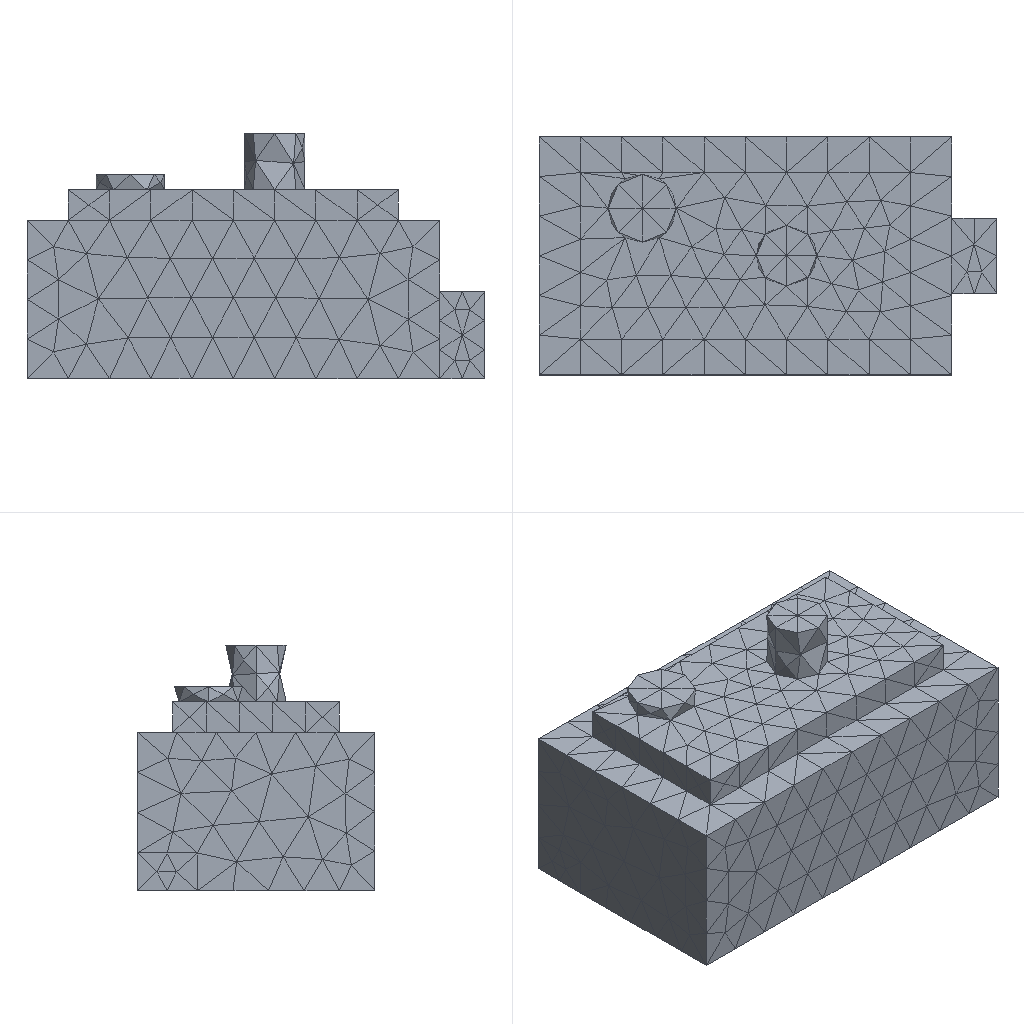Simulation study | ansys mapdl
Set-up summary:
category,name,step,type,value,unit,region
solver,ansys_mapdl
units,mm-N-s-tonne (MPa),,inferred,E=210000 density=
analysis,model,,static
mesh,nodes,,,4621
mesh,elements,,,2783
element_type,SOLID187,,,2783
material,mat 1,,E,210000
material,mat 1,,nu,0.3
load,,model,body load temp,,,all
load,,model,force,"1000 [dir=(0, 0, -1) n=138]",,node list
bc,,model,fixed,"[dofs=UX,UY,UZ n=4927]",,node list
Ansys APDL input file, long lists of numbers shortened:
/COM,ANSYS RELEASE 2026 R1           BUILD 26.1      UP20260202       09:08:46
/PREP7
/NOPR
/TITLE,2
ANTYPE, 0
*IF,_CDRDOFF,EQ,1,THEN     !if solid model was read in
_CDRDOFF=             !reset flag, numoffs already performed
*ELSE              !offset database for the following FE model
NUMOFF,NODE,     4621
NUMOFF,ELEM,     2783
NUMOFF,MAT ,        1
NUMOFF,TYPE,        1
*ENDIF
*SET,_RETURN ,  0.
*SET,_STATUS ,  0.
*SET,_UIQR   ,  138.
*SET,__FLOATPARAMETER__,  4621.
DOF,DELETE
ETBLOCK,        1,        1
(2i9,19a9)
        1      187        0        0        0        0        0        0        0        0        0        0        0        0        0        0        0        0        0        0        0
       -1
NBLOCK,6,SOLID,      4621,      4621
(3i9,6e21.13e3)
        1        0        0-3.8625000000000E+001 3.1500000000000E+001 1.0000000000000E+001
! (4620 more lines like these left out)
N,UNBL,LOC,       -1,
EBLOCK,19,SOLID,      2783,      2783
(19i10)
         1         1         1         1         0         0         0         0        10         0         1      1542      1719       451      1720      1993      1994      1995      1996
! (5565 more lines like these left out)
        -1
MPTEMP,UNBL, 1, 1,  0.    ,
MPDATA,UNBL, 1,EX  ,       1, 1,  210000.000    ,
MPTEMP,UNBL, 1, 1,  0.    ,
MPDATA,UNBL, 1,NUXY,       1, 1, 0.3    ,
MPTEMP,UNBL, 1, 1,  0.    ,
MPDATA,UNBL, 1,PRXY,       1, 1, 0.3    ,
EXTOPT,ATTR,      0,      0,      0
EXTOPT,ESIZE,  0,  0.
EXTOPT,ACLEAR,      0
TREF,  0.
IRLF,  0
BFUNIF,TEMP,_TINY
ACEL,  0.    ,  0.    ,  0.
OMEGA,  0.    ,  0.    ,  0.
DOMEGA,  0.    ,  0.    ,  0.
CGLOC,  0.    ,  0.    ,  0.
CGOMEGA,  0.    ,  0.    ,  0.
DCGOMG,  0.    ,  0.    ,  0.
KUSE,     0
TIME,  0.
ALPHAD,  0.
BETAD,  0.
DMPRAT,  0.
DMPSTR,  0.
CRPLIM, 0.1    ,   0
CRPLIM,  0.    ,   1
NCNV,     0, 1.000000000E+12,     0,  0.    ,  0.
NEQIT,     0
ERESX,DEFA
DBLOCK,      4927
(i9,a6,2(pg16.9))
        1  UX    0.00000000      0.00000000
! (4926 more lines like these left out)
       -1
FBLOCK,       138
(i9,a6,2(pg16.9))
      824  FZ   -7.24637681      0.00000000
! (137 more lines like these left out)
       -1
/GO
FINISH
Results summary:
result,analysis_type_db,,,static,unstated
result,n_sets,,,1,unstated
result,load_steps[0].set,load_step=1,,1,unstated
result,load_steps[0].substep,load_step=1,,1,unstated
result,load_steps[0].time,load_step=1,,1,unstated
result,load_steps[0].freq,load_step=1,,1,unstated
result,load_steps[0].max_usum,load_step=1,,0.0004131,unstated
result,load_steps[0].max_seqv,load_step=1,,4.888,unstated
result,load_steps[0].reaction_sum.FX,load_step=1,,1.0969e-11,unstated
result,load_steps[0].reaction_sum.FY,load_step=1,,-1.69153e-11,unstated
result,load_steps[0].reaction_sum.FZ,load_step=1,,1000,unstated
result,load_steps[0].reaction_sum.MX,load_step=1,,0,unstated
result,load_steps[0].reaction_sum.MY,load_step=1,,0,unstated
result,load_steps[0].reaction_sum.MZ,load_step=1,,0,unstated
result,convergence,,,results present for all listed sets,unstated